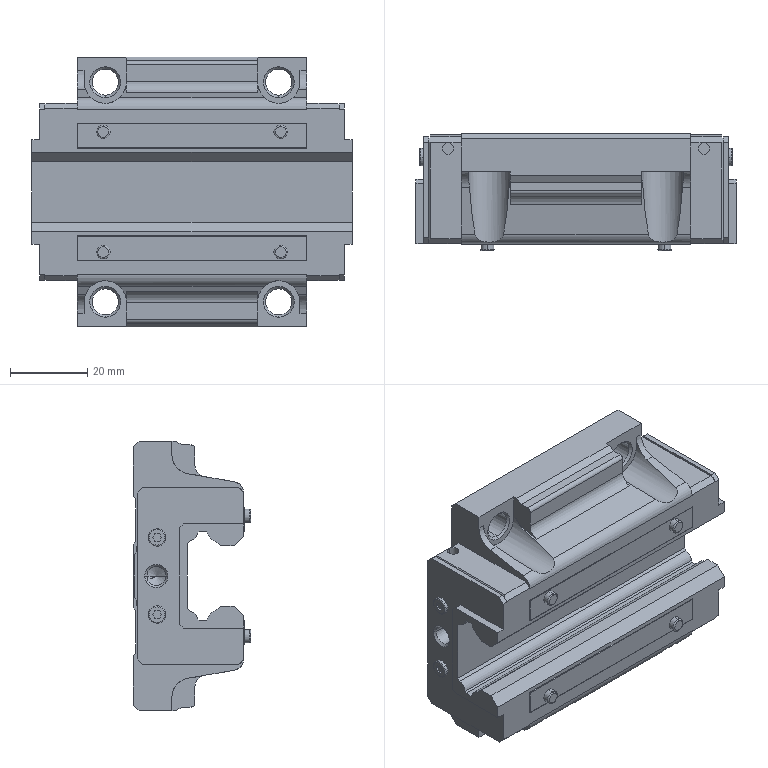Part | SolidWorks | features BaseBody 1 | 1 solid | 284 faces | box 83.1 x 30.5 x 70 mm | volume 101733 mm3 | plane 170 | cylinder 74 | cone 24 | torus 16 | commonest cylinder face diameters 10 x12 3 x8 3.518 x8 4.5 x8 4.917 x8 6.8 x8